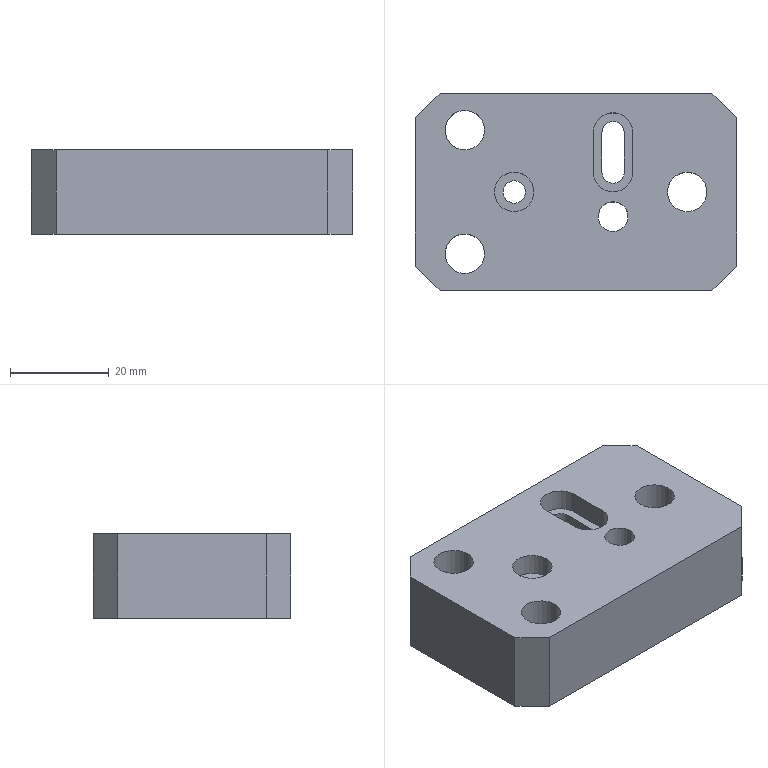Part | SolidWorks | features ICE 4, HoleWzd 3, Chamfer 1, Extrusion 1 | 1 solid | 40 faces | box 65 x 40 x 17 mm | volume 37212 mm3 | cylinder 20 | plane 20 | commonest cylinder face diameters 8 x12 4.5 x4 6 x2 12 x2
STEP:
#1=CARTESIAN_POINT('',(10.5,-5.,8.5));
#2=VERTEX_POINT('',#1);
#3=CARTESIAN_POINT('',(4.5,-5.,8.5));
#4=VERTEX_POINT('',#3);
#5=CARTESIAN_POINT('',(7.5,-5.,8.5));
#6=DIRECTION('',(0.,0.,-1.));
#7=DIRECTION('',(-1.,0.,0.));
#8=AXIS2_PLACEMENT_3D('',#5,#6,#7);
#9=CIRCLE('',#8,3.);
#10=EDGE_CURVE('',#2,#4,#9,.T.);
#11=ORIENTED_EDGE('',*,*,#10,.F.);
#12=CARTESIAN_POINT('',(10.5,-5.,-8.5));
#13=VERTEX_POINT('',#12);
#14=CARTESIAN_POINT('',(10.5,-5.,-8.5));
#15=DIRECTION('',(0.,0.,-1.));
#16=VECTOR('',#15,1000.);
#17=LINE('',#14,#16);
#18=EDGE_CURVE('',#2,#13,#17,.T.);
#19=ORIENTED_EDGE('',*,*,#18,.T.);
#20=CARTESIAN_POINT('',(4.5,-5.,-8.5));
#21=VERTEX_POINT('',#20);
#22=CARTESIAN_POINT('',(7.5,-5.,-8.5));
#23=DIRECTION('',(0.,0.,-1.));
#24=DIRECTION('',(-1.,0.,0.));
#25=AXIS2_PLACEMENT_3D('',#22,#23,#24);
#26=CIRCLE('',#25,3.);
#27=EDGE_CURVE('',#13,#21,#26,.T.);
#28=ORIENTED_EDGE('',*,*,#27,.T.);
#29=CARTESIAN_POINT('',(4.5,-5.,-8.5));
#30=DIRECTION('',(0.,0.,-1.));
#31=VECTOR('',#30,1000.);
#32=LINE('',#29,#31);
#33=EDGE_CURVE('',#4,#21,#32,.T.);
#34=ORIENTED_EDGE('',*,*,#33,.F.);
#35=EDGE_LOOP('',(#11,#19,#28,#34));
#36=FACE_OUTER_BOUND('',#35,.T.);
#37=CARTESIAN_POINT('',(7.5,-5.,-8.5));
#38=DIRECTION('',(0.,0.,-1.));
#39=DIRECTION('',(-1.,0.,0.));
#40=AXIS2_PLACEMENT_3D('',#37,#38,#39);
#41=CYLINDRICAL_SURFACE('',#40,3.);
#42=ADVANCED_FACE('',(#36),#41,.F.);
#43=CARTESIAN_POINT('',(-16.5,0.,4.1));
#44=VERTEX_POINT('',#43);
#45=CARTESIAN_POINT('',(-8.5,0.,4.1));
#46=VERTEX_POINT('',#45);
#47=CARTESIAN_POINT('',(-12.5,0.,4.1));
#48=DIRECTION('',(0.,0.,1.));
#49=DIRECTION('',(1.,0.,0.));
#50=AXIS2_PLACEMENT_3D('',#47,#48,#49);
#51=CIRCLE('',#50,4.);
#52=EDGE_CURVE('',#44,#46,#51,.T.);
#53=ORIENTED_EDGE('',*,*,#52,.F.);
#54=CARTESIAN_POINT('',(-16.5,0.,8.5));
#55=VERTEX_POINT('',#54);
#56=CARTESIAN_POINT('',(-16.5,0.,8.5));
#57=DIRECTION('',(0.,0.,1.));
#58=VECTOR('',#57,1000.);
#59=LINE('',#56,#58);
#60=EDGE_CURVE('',#44,#55,#59,.T.);
#61=ORIENTED_EDGE('',*,*,#60,.T.);
#62=CARTESIAN_POINT('',(-8.5,0.,8.5));
#63=VERTEX_POINT('',#62);
#64=CARTESIAN_POINT('',(-12.5,0.,8.5));
#65=DIRECTION('',(0.,0.,1.));
#66=DIRECTION('',(1.,0.,0.));
#67=AXIS2_PLACEMENT_3D('',#64,#65,#66);
#68=CIRCLE('',#67,4.);
#69=EDGE_CURVE('',#55,#63,#68,.T.);
#70=ORIENTED_EDGE('',*,*,#69,.T.);
#71=CARTESIAN_POINT('',(-8.5,0.,8.5));
#72=DIRECTION('',(0.,0.,1.));
#73=VECTOR('',#72,1000.);
#74=LINE('',#71,#73);
#75=EDGE_CURVE('',#46,#63,#74,.T.);
#76=ORIENTED_EDGE('',*,*,#75,.F.);
#77=EDGE_LOOP('',(#53,#61,#70,#76));
#78=FACE_OUTER_BOUND('',#77,.T.);
#79=CARTESIAN_POINT('',(-12.5,0.,8.5));
#80=DIRECTION('',(0.,0.,1.));
#81=DIRECTION('',(1.,0.,0.));
#82=AXIS2_PLACEMENT_3D('',#79,#80,#81);
#83=CYLINDRICAL_SURFACE('',#82,4.);
#84=ADVANCED_FACE('',(#78),#83,.F.);
#85=CARTESIAN_POINT('',(-10.25,0.,1.));
#86=VERTEX_POINT('',#85);
#87=CARTESIAN_POINT('',(-14.75,0.,1.));
#88=VERTEX_POINT('',#87);
#89=CARTESIAN_POINT('',(-12.5,0.,1.));
#90=DIRECTION('',(0.,0.,-1.));
#91=DIRECTION('',(-1.,0.,0.));
#92=AXIS2_PLACEMENT_3D('',#89,#90,#91);
#93=CIRCLE('',#92,2.25);
#94=EDGE_CURVE('',#86,#88,#93,.T.);
#95=ORIENTED_EDGE('',*,*,#94,.T.);
#96=CARTESIAN_POINT('',(-14.75,0.,4.1));
#97=VERTEX_POINT('',#96);
#98=CARTESIAN_POINT('',(-14.75,0.,8.5));
#99=DIRECTION('',(0.,0.,1.));
#100=VECTOR('',#99,1000.);
#101=LINE('',#98,#100);
#102=EDGE_CURVE('',#88,#97,#101,.T.);
#103=ORIENTED_EDGE('',*,*,#102,.T.);
#104=CARTESIAN_POINT('',(-10.25,0.,4.1));
#105=VERTEX_POINT('',#104);
#106=CARTESIAN_POINT('',(-12.5,0.,4.1));
#107=DIRECTION('',(0.,0.,1.));
#108=DIRECTION('',(1.,0.,0.));
#109=AXIS2_PLACEMENT_3D('',#106,#107,#108);
#110=CIRCLE('',#109,2.25);
#111=EDGE_CURVE('',#97,#105,#110,.T.);
#112=ORIENTED_EDGE('',*,*,#111,.T.);
#113=CARTESIAN_POINT('',(-10.25,0.,8.5));
#114=DIRECTION('',(0.,0.,1.));
#115=VECTOR('',#114,1000.);
#116=LINE('',#113,#115);
#117=EDGE_CURVE('',#86,#105,#116,.T.);
#118=ORIENTED_EDGE('',*,*,#117,.F.);
#119=EDGE_LOOP('',(#95,#103,#112,#118));
#120=FACE_OUTER_BOUND('',#119,.T.);
#121=CARTESIAN_POINT('',(-12.5,0.,8.5));
#122=DIRECTION('',(0.,0.,1.));
#123=DIRECTION('',(1.,0.,0.));
#124=AXIS2_PLACEMENT_3D('',#121,#122,#123);
#125=CYLINDRICAL_SURFACE('',#124,2.25);
#126=ADVANCED_FACE('',(#120),#125,.F.);
#127=CARTESIAN_POINT('',(-6.5,0.,1.));
#128=VERTEX_POINT('',#127);
#129=CARTESIAN_POINT('',(-18.5,0.,1.));
#130=VERTEX_POINT('',#129);
#131=CARTESIAN_POINT('',(-12.5,0.,1.));
#132=DIRECTION('',(0.,0.,-1.));
#133=DIRECTION('',(-1.,0.,0.));
#134=AXIS2_PLACEMENT_3D('',#131,#132,#133);
#135=CIRCLE('',#134,6.);
#136=EDGE_CURVE('',#128,#130,#135,.T.);
#137=ORIENTED_EDGE('',*,*,#136,.F.);
#138=CARTESIAN_POINT('',(-6.5,0.,-8.5));
#139=VERTEX_POINT('',#138);
#140=CARTESIAN_POINT('',(-6.5,0.,1.));
#141=DIRECTION('',(0.,0.,-1.));
#142=VECTOR('',#141,1000.);
#143=LINE('',#140,#142);
#144=EDGE_CURVE('',#128,#139,#143,.T.);
#145=ORIENTED_EDGE('',*,*,#144,.T.);
#146=CARTESIAN_POINT('',(-18.5,0.,-8.5));
#147=VERTEX_POINT('',#146);
#148=CARTESIAN_POINT('',(-12.5,0.,-8.5));
#149=DIRECTION('',(0.,0.,-1.));
#150=DIRECTION('',(-1.,0.,0.));
#151=AXIS2_PLACEMENT_3D('',#148,#149,#150);
#152=CIRCLE('',#151,6.);
#153=EDGE_CURVE('',#139,#147,#152,.T.);
#154=ORIENTED_EDGE('',*,*,#153,.T.);
#155=CARTESIAN_POINT('',(-18.5,0.,1.));
#156=DIRECTION('',(0.,0.,-1.));
#157=VECTOR('',#156,1000.);
#158=LINE('',#155,#157);
#159=EDGE_CURVE('',#130,#147,#158,.T.);
#160=ORIENTED_EDGE('',*,*,#159,.F.);
#161=EDGE_LOOP('',(#137,#145,#154,#160));
#162=FACE_OUTER_BOUND('',#161,.T.);
#163=CARTESIAN_POINT('',(-12.5,0.,1.));
#164=DIRECTION('',(0.,0.,-1.));
#165=DIRECTION('',(-1.,0.,0.));
#166=AXIS2_PLACEMENT_3D('',#163,#164,#165);
#167=CYLINDRICAL_SURFACE('',#166,6.);
#168=ADVANCED_FACE('',(#162),#167,.F.);
#169=CARTESIAN_POINT('',(-26.5,12.5,-8.5));
#170=VERTEX_POINT('',#169);
#171=CARTESIAN_POINT('',(-18.5,12.5,-8.5));
#172=VERTEX_POINT('',#171);
#173=CARTESIAN_POINT('',(-22.5,12.5,-8.5));
#174=DIRECTION('',(0.,0.,1.));
#175=DIRECTION('',(1.,0.,0.));
#176=AXIS2_PLACEMENT_3D('',#173,#174,#175);
#177=CIRCLE('',#176,4.);
#178=EDGE_CURVE('',#170,#172,#177,.T.);
#179=ORIENTED_EDGE('',*,*,#178,.F.);
#180=CARTESIAN_POINT('',(-26.5,12.5,8.5));
#181=VERTEX_POINT('',#180);
#182=CARTESIAN_POINT('',(-26.5,12.5,8.5));
#183=DIRECTION('',(0.,0.,1.));
#184=VECTOR('',#183,1000.);
#185=LINE('',#182,#184);
#186=EDGE_CURVE('',#170,#181,#185,.T.);
#187=ORIENTED_EDGE('',*,*,#186,.T.);
#188=CARTESIAN_POINT('',(-18.5,12.5,8.5));
#189=VERTEX_POINT('',#188);
#190=CARTESIAN_POINT('',(-22.5,12.5,8.5));
#191=DIRECTION('',(0.,0.,1.));
#192=DIRECTION('',(1.,0.,0.));
#193=AXIS2_PLACEMENT_3D('',#190,#191,#192);
#194=CIRCLE('',#193,4.);
#195=EDGE_CURVE('',#181,#189,#194,.T.);
#196=ORIENTED_EDGE('',*,*,#195,.T.);
#197=CARTESIAN_POINT('',(-18.5,12.5,8.5));
#198=DIRECTION('',(0.,0.,1.));
#199=VECTOR('',#198,1000.);
#200=LINE('',#197,#199);
#201=EDGE_CURVE('',#172,#189,#200,.T.);
#202=ORIENTED_EDGE('',*,*,#201,.F.);
#203=EDGE_LOOP('',(#179,#187,#196,#202));
#204=FACE_OUTER_BOUND('',#203,.T.);
#205=CARTESIAN_POINT('',(-22.5,12.5,8.5));
#206=DIRECTION('',(0.,0.,1.));
#207=DIRECTION('',(1.,0.,0.));
#208=AXIS2_PLACEMENT_3D('',#205,#206,#207);
#209=CYLINDRICAL_SURFACE('',#208,4.);
#210=ADVANCED_FACE('',(#204),#209,.F.);
#211=CARTESIAN_POINT('',(-26.5,-12.5,-8.5));
#212=VERTEX_POINT('',#211);
#213=CARTESIAN_POINT('',(-18.5,-12.5,-8.5));
#214=VERTEX_POINT('',#213);
#215=CARTESIAN_POINT('',(-22.5,-12.5,-8.5));
#216=DIRECTION('',(0.,0.,1.));
#217=DIRECTION('',(1.,0.,0.));
#218=AXIS2_PLACEMENT_3D('',#215,#216,#217);
#219=CIRCLE('',#218,4.);
#220=EDGE_CURVE('',#212,#214,#219,.T.);
#221=ORIENTED_EDGE('',*,*,#220,.F.);
#222=CARTESIAN_POINT('',(-26.5,-12.5,8.5));
#223=VERTEX_POINT('',#222);
#224=CARTESIAN_POINT('',(-26.5,-12.5,8.5));
#225=DIRECTION('',(0.,0.,1.));
#226=VECTOR('',#225,1000.);
#227=LINE('',#224,#226);
#228=EDGE_CURVE('',#212,#223,#227,.T.);
#229=ORIENTED_EDGE('',*,*,#228,.T.);
#230=CARTESIAN_POINT('',(-18.5,-12.5,8.5));
#231=VERTEX_POINT('',#230);
#232=CARTESIAN_POINT('',(-22.5,-12.5,8.5));
#233=DIRECTION('',(0.,0.,1.));
#234=DIRECTION('',(1.,0.,0.));
#235=AXIS2_PLACEMENT_3D('',#232,#233,#234);
#236=CIRCLE('',#235,4.);
#237=EDGE_CURVE('',#223,#231,#236,.T.);
#238=ORIENTED_EDGE('',*,*,#237,.T.);
#239=CARTESIAN_POINT('',(-18.5,-12.5,8.5));
#240=DIRECTION('',(0.,0.,1.));
#241=VECTOR('',#240,1000.);
#242=LINE('',#239,#241);
#243=EDGE_CURVE('',#214,#231,#242,.T.);
#244=ORIENTED_EDGE('',*,*,#243,.F.);
#245=EDGE_LOOP('',(#221,#229,#238,#244));
#246=FACE_OUTER_BOUND('',#245,.T.);
#247=CARTESIAN_POINT('',(-22.5,-12.5,8.5));
#248=DIRECTION('',(0.,0.,1.));
#249=DIRECTION('',(1.,0.,0.));
#250=AXIS2_PLACEMENT_3D('',#247,#248,#249);
#251=CYLINDRICAL_SURFACE('',#250,4.);
#252=ADVANCED_FACE('',(#246),#251,.F.);
#253=CARTESIAN_POINT('',(18.5,0.,-8.5));
#254=VERTEX_POINT('',#253);
#255=CARTESIAN_POINT('',(26.5,0.,-8.5));
#256=VERTEX_POINT('',#255);
#257=CARTESIAN_POINT('',(22.5,0.,-8.5));
#258=DIRECTION('',(0.,0.,1.));
#259=DIRECTION('',(1.,0.,0.));
#260=AXIS2_PLACEMENT_3D('',#257,#258,#259);
#261=CIRCLE('',#260,4.);
#262=EDGE_CURVE('',#254,#256,#261,.T.);
#263=ORIENTED_EDGE('',*,*,#262,.F.);
#264=CARTESIAN_POINT('',(18.5,0.,8.5));
#265=VERTEX_POINT('',#264);
#266=CARTESIAN_POINT('',(18.5,0.,8.5));
#267=DIRECTION('',(0.,0.,1.));
#268=VECTOR('',#267,1000.);
#269=LINE('',#266,#268);
#270=EDGE_CURVE('',#254,#265,#269,.T.);
#271=ORIENTED_EDGE('',*,*,#270,.T.);
#272=CARTESIAN_POINT('',(26.5,0.,8.5));
#273=VERTEX_POINT('',#272);
#274=CARTESIAN_POINT('',(22.5,0.,8.5));
#275=DIRECTION('',(0.,0.,1.));
#276=DIRECTION('',(1.,0.,0.));
#277=AXIS2_PLACEMENT_3D('',#274,#275,#276);
#278=CIRCLE('',#277,4.);
#279=EDGE_CURVE('',#265,#273,#278,.T.);
#280=ORIENTED_EDGE('',*,*,#279,.T.);
#281=CARTESIAN_POINT('',(26.5,0.,8.5));
#282=DIRECTION('',(0.,0.,1.));
#283=VECTOR('',#282,1000.);
#284=LINE('',#281,#283);
#285=EDGE_CURVE('',#256,#273,#284,.T.);
#286=ORIENTED_EDGE('',*,*,#285,.F.);
#287=EDGE_LOOP('',(#263,#271,#280,#286));
#288=FACE_OUTER_BOUND('',#287,.T.);
#289=CARTESIAN_POINT('',(22.5,0.,8.5));
#290=DIRECTION('',(0.,0.,1.));
#291=DIRECTION('',(1.,0.,0.));
#292=AXIS2_PLACEMENT_3D('',#289,#290,#291);
#293=CYLINDRICAL_SURFACE('',#292,4.);
#294=ADVANCED_FACE('',(#288),#293,.F.);
#295=CARTESIAN_POINT('',(32.5,-15.,-8.5));
#296=VERTEX_POINT('',#295);
#297=CARTESIAN_POINT('',(32.5,15.,-8.5));
#298=VERTEX_POINT('',#297);
#299=CARTESIAN_POINT('',(32.5,-20.,-8.5));
#300=DIRECTION('',(0.,1.,0.));
#301=VECTOR('',#300,1000.);
#302=LINE('',#299,#301);
#303=EDGE_CURVE('',#296,#298,#302,.T.);
#304=ORIENTED_EDGE('',*,*,#303,.T.);
#305=CARTESIAN_POINT('',(32.5,15.,8.5));
#306=VERTEX_POINT('',#305);
#307=CARTESIAN_POINT('',(32.5,15.,8.5));
#308=DIRECTION('',(0.,0.,1.));
#309=VECTOR('',#308,1000.);
#310=LINE('',#307,#309);
#311=EDGE_CURVE('',#298,#306,#310,.T.);
#312=ORIENTED_EDGE('',*,*,#311,.T.);
#313=CARTESIAN_POINT('',(32.5,-15.,8.5));
#314=VERTEX_POINT('',#313);
#315=CARTESIAN_POINT('',(32.5,-20.,8.5));
#316=DIRECTION('',(0.,1.,0.));
#317=VECTOR('',#316,1000.);
#318=LINE('',#315,#317);
#319=EDGE_CURVE('',#314,#306,#318,.T.);
#320=ORIENTED_EDGE('',*,*,#319,.F.);
#321=CARTESIAN_POINT('',(32.5,-15.,8.5));
#322=DIRECTION('',(0.,0.,-1.));
#323=VECTOR('',#322,1000.);
#324=LINE('',#321,#323);
#325=EDGE_CURVE('',#314,#296,#324,.T.);
#326=ORIENTED_EDGE('',*,*,#325,.T.);
#327=EDGE_LOOP('',(#304,#312,#320,#326));
#328=FACE_OUTER_BOUND('',#327,.T.);
#329=CARTESIAN_POINT('',(32.5,-20.,8.5));
#330=DIRECTION('',(-1.,0.,0.));
#331=DIRECTION('',(0.,0.,1.));
#332=AXIS2_PLACEMENT_3D('',#329,#330,#331);
#333=PLANE('',#332);
#334=ADVANCED_FACE('',(#328),#333,.F.);
#335=CARTESIAN_POINT('',(27.5,20.,-8.5));
#336=VERTEX_POINT('',#335);
#337=CARTESIAN_POINT('',(-27.5,20.,-8.5));
#338=VERTEX_POINT('',#337);
#339=CARTESIAN_POINT('',(-32.5,20.,-8.5));
#340=DIRECTION('',(-1.,0.,0.));
#341=VECTOR('',#340,1000.);
#342=LINE('',#339,#341);
#343=EDGE_CURVE('',#336,#338,#342,.T.);
#344=ORIENTED_EDGE('',*,*,#343,.T.);
#345=CARTESIAN_POINT('',(-27.5,20.,8.5));
#346=VERTEX_POINT('',#345);
#347=CARTESIAN_POINT('',(-27.5,20.,8.5));
#348=DIRECTION('',(0.,0.,1.));
#349=VECTOR('',#348,1000.);
#350=LINE('',#347,#349);
#351=EDGE_CURVE('',#338,#346,#350,.T.);
#352=ORIENTED_EDGE('',*,*,#351,.T.);
#353=CARTESIAN_POINT('',(27.5,20.,8.5));
#354=VERTEX_POINT('',#353);
#355=CARTESIAN_POINT('',(-32.5,20.,8.5));
#356=DIRECTION('',(-1.,0.,0.));
#357=VECTOR('',#356,1000.);
#358=LINE('',#355,#357);
#359=EDGE_CURVE('',#354,#346,#358,.T.);
#360=ORIENTED_EDGE('',*,*,#359,.F.);
#361=CARTESIAN_POINT('',(27.5,20.,8.5));
#362=DIRECTION('',(0.,0.,-1.));
#363=VECTOR('',#362,1000.);
#364=LINE('',#361,#363);
#365=EDGE_CURVE('',#354,#336,#364,.T.);
#366=ORIENTED_EDGE('',*,*,#365,.T.);
#367=EDGE_LOOP('',(#344,#352,#360,#366));
#368=FACE_OUTER_BOUND('',#367,.T.);
#369=CARTESIAN_POINT('',(-32.5,20.,8.5));
#370=DIRECTION('',(0.,-1.,0.));
#371=DIRECTION('',(0.,0.,-1.));
#372=AXIS2_PLACEMENT_3D('',#369,#370,#371);
#373=PLANE('',#372);
#374=ADVANCED_FACE('',(#368),#373,.F.);
#375=CARTESIAN_POINT('',(-32.5,15.,-8.5));
#376=VERTEX_POINT('',#375);
#377=CARTESIAN_POINT('',(-32.5,-15.,-8.5));
#378=VERTEX_POINT('',#377);
#379=CARTESIAN_POINT('',(-32.5,-20.,-8.5));
#380=DIRECTION('',(0.,-1.,0.));
#381=VECTOR('',#380,1000.);
#382=LINE('',#379,#381);
#383=EDGE_CURVE('',#376,#378,#382,.T.);
#384=ORIENTED_EDGE('',*,*,#383,.T.);
#385=CARTESIAN_POINT('',(-32.5,-15.,8.5));
#386=VERTEX_POINT('',#385);
#387=CARTESIAN_POINT('',(-32.5,-15.,8.5));
#388=DIRECTION('',(0.,0.,1.));
#389=VECTOR('',#388,1000.);
#390=LINE('',#387,#389);
#391=EDGE_CURVE('',#378,#386,#390,.T.);
#392=ORIENTED_EDGE('',*,*,#391,.T.);
#393=CARTESIAN_POINT('',(-32.5,15.,8.5));
#394=VERTEX_POINT('',#393);
#395=CARTESIAN_POINT('',(-32.5,-20.,8.5));
#396=DIRECTION('',(0.,-1.,0.));
#397=VECTOR('',#396,1000.);
#398=LINE('',#395,#397);
#399=EDGE_CURVE('',#394,#386,#398,.T.);
#400=ORIENTED_EDGE('',*,*,#399,.F.);
#401=CARTESIAN_POINT('',(-32.5,15.,8.5));
#402=DIRECTION('',(0.,0.,-1.));
#403=VECTOR('',#402,1000.);
#404=LINE('',#401,#403);
#405=EDGE_CURVE('',#394,#376,#404,.T.);
#406=ORIENTED_EDGE('',*,*,#405,.T.);
#407=EDGE_LOOP('',(#384,#392,#400,#406));
#408=FACE_OUTER_BOUND('',#407,.T.);
#409=CARTESIAN_POINT('',(-32.5,-20.,8.5));
#410=DIRECTION('',(1.,0.,0.));
#411=DIRECTION('',(0.,0.,-1.));
#412=AXIS2_PLACEMENT_3D('',#409,#410,#411);
#413=PLANE('',#412);
#414=ADVANCED_FACE('',(#408),#413,.F.);
#415=CARTESIAN_POINT('',(-27.5,-20.,8.5));
#416=VERTEX_POINT('',#415);
#417=CARTESIAN_POINT('',(27.5,-20.,8.5));
#418=VERTEX_POINT('',#417);
#419=CARTESIAN_POINT('',(-32.5,-20.,8.5));
#420=DIRECTION('',(1.,0.,0.));
#421=VECTOR('',#420,1000.);
#422=LINE('',#419,#421);
#423=EDGE_CURVE('',#416,#418,#422,.T.);
#424=ORIENTED_EDGE('',*,*,#423,.F.);
#425=CARTESIAN_POINT('',(-27.5,-20.,-8.5));
#426=VERTEX_POINT('',#425);
#427=CARTESIAN_POINT('',(-27.5,-20.,8.5));
#428=DIRECTION('',(0.,0.,-1.));
#429=VECTOR('',#428,1000.);
#430=LINE('',#427,#429);
#431=EDGE_CURVE('',#416,#426,#430,.T.);
#432=ORIENTED_EDGE('',*,*,#431,.T.);
#433=CARTESIAN_POINT('',(27.5,-20.,-8.5));
#434=VERTEX_POINT('',#433);
#435=CARTESIAN_POINT('',(-32.5,-20.,-8.5));
#436=DIRECTION('',(1.,0.,0.));
#437=VECTOR('',#436,1000.);
#438=LINE('',#435,#437);
#439=EDGE_CURVE('',#426,#434,#438,.T.);
#440=ORIENTED_EDGE('',*,*,#439,.T.);
#441=CARTESIAN_POINT('',(27.5,-20.,8.5));
#442=DIRECTION('',(0.,0.,1.));
#443=VECTOR('',#442,1000.);
#444=LINE('',#441,#443);
#445=EDGE_CURVE('',#434,#418,#444,.T.);
#446=ORIENTED_EDGE('',*,*,#445,.T.);
#447=EDGE_LOOP('',(#424,#432,#440,#446));
#448=FACE_OUTER_BOUND('',#447,.T.);
#449=CARTESIAN_POINT('',(-32.5,-20.,8.5));
#450=DIRECTION('',(0.,1.,0.));
#451=DIRECTION('',(0.,0.,1.));
#452=AXIS2_PLACEMENT_3D('',#449,#450,#451);
#453=PLANE('',#452);
#454=ADVANCED_FACE('',(#448),#453,.F.);
#455=CARTESIAN_POINT('',(11.5,12.,8.5));
#456=VERTEX_POINT('',#455);
#457=CARTESIAN_POINT('',(3.5,12.,8.5));
#458=VERTEX_POINT('',#457);
#459=CARTESIAN_POINT('',(7.5,12.,8.5));
#460=DIRECTION('',(0.,0.,1.));
#461=DIRECTION('',(1.,0.,0.));
#462=AXIS2_PLACEMENT_3D('',#459,#460,#461);
#463=CIRCLE('',#462,4.);
#464=EDGE_CURVE('',#456,#458,#463,.T.);
#465=ORIENTED_EDGE('',*,*,#464,.F.);
#466=CARTESIAN_POINT('',(11.5,4.,8.5));
#467=VERTEX_POINT('',#466);
#468=CARTESIAN_POINT('',(11.5,4.,8.5));
#469=DIRECTION('',(0.,1.,0.));
#470=VECTOR('',#469,1000.);
#471=LINE('',#468,#470);
#472=EDGE_CURVE('',#467,#456,#471,.T.);
#473=ORIENTED_EDGE('',*,*,#472,.F.);
#474=CARTESIAN_POINT('',(3.5,4.,8.5));
#475=VERTEX_POINT('',#474);
#476=CARTESIAN_POINT('',(7.5,4.,8.5));
#477=DIRECTION('',(0.,0.,1.));
#478=DIRECTION('',(1.,0.,0.));
#479=AXIS2_PLACEMENT_3D('',#476,#477,#478);
#480=CIRCLE('',#479,4.);
#481=EDGE_CURVE('',#475,#467,#480,.T.);
#482=ORIENTED_EDGE('',*,*,#481,.F.);
#483=CARTESIAN_POINT('',(3.5,4.,8.5));
#484=DIRECTION('',(0.,-1.,0.));
#485=VECTOR('',#484,1000.);
#486=LINE('',#483,#485);
#487=EDGE_CURVE('',#458,#475,#486,.T.);
#488=ORIENTED_EDGE('',*,*,#487,.F.);
#489=EDGE_LOOP('',(#465,#473,#482,#488));
#490=FACE_BOUND('',#489,.T.);
#491=CARTESIAN_POINT('',(7.5,-5.,8.5));
#492=DIRECTION('',(0.,0.,-1.));
#493=DIRECTION('',(-1.,0.,0.));
#494=AXIS2_PLACEMENT_3D('',#491,#492,#493);
#495=CIRCLE('',#494,3.);
#496=EDGE_CURVE('',#4,#2,#495,.T.);
#497=ORIENTED_EDGE('',*,*,#496,.T.);
#498=ORIENTED_EDGE('',*,*,#10,.T.);
#499=EDGE_LOOP('',(#497,#498));
#500=FACE_BOUND('',#499,.T.);
#501=CARTESIAN_POINT('',(-12.5,0.,8.5));
#502=DIRECTION('',(0.,0.,1.));
#503=DIRECTION('',(1.,0.,0.));
#504=AXIS2_PLACEMENT_3D('',#501,#502,#503);
#505=CIRCLE('',#504,4.);
#506=EDGE_CURVE('',#63,#55,#505,.T.);
#507=ORIENTED_EDGE('',*,*,#506,.F.);
#508=ORIENTED_EDGE('',*,*,#69,.F.);
#509=EDGE_LOOP('',(#507,#508));
#510=FACE_BOUND('',#509,.T.);
#511=CARTESIAN_POINT('',(-22.5,12.5,8.5));
#512=DIRECTION('',(0.,0.,1.));
#513=DIRECTION('',(1.,0.,0.));
#514=AXIS2_PLACEMENT_3D('',#511,#512,#513);
#515=CIRCLE('',#514,4.);
#516=EDGE_CURVE('',#189,#181,#515,.T.);
#517=ORIENTED_EDGE('',*,*,#516,.F.);
#518=ORIENTED_EDGE('',*,*,#195,.F.);
#519=EDGE_LOOP('',(#517,#518));
#520=FACE_BOUND('',#519,.T.);
#521=CARTESIAN_POINT('',(-22.5,-12.5,8.5));
#522=DIRECTION('',(0.,0.,1.));
#523=DIRECTION('',(1.,0.,0.));
#524=AXIS2_PLACEMENT_3D('',#521,#522,#523);
#525=CIRCLE('',#524,4.);
#526=EDGE_CURVE('',#231,#223,#525,.T.);
#527=ORIENTED_EDGE('',*,*,#526,.F.);
#528=ORIENTED_EDGE('',*,*,#237,.F.);
#529=EDGE_LOOP('',(#527,#528));
#530=FACE_BOUND('',#529,.T.);
#531=CARTESIAN_POINT('',(22.5,0.,8.5));
#532=DIRECTION('',(0.,0.,1.));
#533=DIRECTION('',(1.,0.,0.));
#534=AXIS2_PLACEMENT_3D('',#531,#532,#533);
#535=CIRCLE('',#534,4.);
#536=EDGE_CURVE('',#273,#265,#535,.T.);
#537=ORIENTED_EDGE('',*,*,#536,.F.);
#538=ORIENTED_EDGE('',*,*,#279,.F.);
#539=EDGE_LOOP('',(#537,#538));
#540=FACE_BOUND('',#539,.T.);
#541=ORIENTED_EDGE('',*,*,#399,.T.);
#542=CARTESIAN_POINT('',(-27.5,-20.,8.5));
#543=DIRECTION('',(0.7071,-0.7071,0.));
#544=VECTOR('',#543,1000.);
#545=LINE('',#542,#544);
#546=EDGE_CURVE('',#386,#416,#545,.T.);
#547=ORIENTED_EDGE('',*,*,#546,.T.);
#548=ORIENTED_EDGE('',*,*,#423,.T.);
#549=CARTESIAN_POINT('',(32.5,-15.,8.5));
#550=DIRECTION('',(0.7071,0.7071,0.));
#551=VECTOR('',#550,1000.);
#552=LINE('',#549,#551);
#553=EDGE_CURVE('',#418,#314,#552,.T.);
#554=ORIENTED_EDGE('',*,*,#553,.T.);
#555=ORIENTED_EDGE('',*,*,#319,.T.);
#556=CARTESIAN_POINT('',(27.5,20.,8.5));
#557=DIRECTION('',(-0.7071,0.7071,0.));
#558=VECTOR('',#557,1000.);
#559=LINE('',#556,#558);
#560=EDGE_CURVE('',#306,#354,#559,.T.);
#561=ORIENTED_EDGE('',*,*,#560,.T.);
#562=ORIENTED_EDGE('',*,*,#359,.T.);
#563=CARTESIAN_POINT('',(-32.5,15.,8.5));
#564=DIRECTION('',(-0.7071,-0.7071,0.));
#565=VECTOR('',#564,1000.);
#566=LINE('',#563,#565);
#567=EDGE_CURVE('',#346,#394,#566,.T.);
#568=ORIENTED_EDGE('',*,*,#567,.T.);
#569=EDGE_LOOP('',(#541,#547,#548,#554,#555,#561,#562,#568));
#570=FACE_OUTER_BOUND('',#569,.T.);
#571=CARTESIAN_POINT('',(0.,0.,8.5));
#572=DIRECTION('',(0.,0.,-1.));
#573=DIRECTION('',(-1.,0.,0.));
#574=AXIS2_PLACEMENT_3D('',#571,#572,#573);
#575=PLANE('',#574);
#576=ADVANCED_FACE('',(#490,#500,#510,#520,#530,#540,#570),#575,.F.);
#577=CARTESIAN_POINT('',(11.5,4.,-8.5));
#578=VERTEX_POINT('',#577);
#579=CARTESIAN_POINT('',(3.5,4.,-8.5));
#580=VERTEX_POINT('',#579);
#581=CARTESIAN_POINT('',(7.5,4.,-8.5));
#582=DIRECTION('',(0.,0.,-1.));
#583=DIRECTION('',(-1.,0.,0.));
#584=AXIS2_PLACEMENT_3D('',#581,#582,#583);
#585=CIRCLE('',#584,4.);
#586=EDGE_CURVE('',#578,#580,#585,.T.);
#587=ORIENTED_EDGE('',*,*,#586,.F.);
#588=CARTESIAN_POINT('',(11.5,12.,-8.5));
#589=VERTEX_POINT('',#588);
#590=CARTESIAN_POINT('',(11.5,4.,-8.5));
#591=DIRECTION('',(0.,-1.,0.));
#592=VECTOR('',#591,1000.);
#593=LINE('',#590,#592);
#594=EDGE_CURVE('',#589,#578,#593,.T.);
#595=ORIENTED_EDGE('',*,*,#594,.F.);
#596=CARTESIAN_POINT('',(3.5,12.,-8.5));
#597=VERTEX_POINT('',#596);
#598=CARTESIAN_POINT('',(7.5,12.,-8.5));
#599=DIRECTION('',(0.,0.,-1.));
#600=DIRECTION('',(-1.,0.,0.));
#601=AXIS2_PLACEMENT_3D('',#598,#599,#600);
#602=CIRCLE('',#601,4.);
#603=EDGE_CURVE('',#597,#589,#602,.T.);
#604=ORIENTED_EDGE('',*,*,#603,.F.);
#605=CARTESIAN_POINT('',(3.5,4.,-8.5));
#606=DIRECTION('',(0.,1.,0.));
#607=VECTOR('',#606,1000.);
#608=LINE('',#605,#607);
#609=EDGE_CURVE('',#580,#597,#608,.T.);
#610=ORIENTED_EDGE('',*,*,#609,.F.);
#611=EDGE_LOOP('',(#587,#595,#604,#610));
#612=FACE_BOUND('',#611,.T.);
#613=CARTESIAN_POINT('',(7.5,-5.,-8.5));
#614=DIRECTION('',(0.,0.,-1.));
#615=DIRECTION('',(-1.,0.,0.));
#616=AXIS2_PLACEMENT_3D('',#613,#614,#615);
#617=CIRCLE('',#616,3.);
#618=EDGE_CURVE('',#21,#13,#617,.T.);
#619=ORIENTED_EDGE('',*,*,#618,.F.);
#620=ORIENTED_EDGE('',*,*,#27,.F.);
#621=EDGE_LOOP('',(#619,#620));
#622=FACE_BOUND('',#621,.T.);
#623=CARTESIAN_POINT('',(-12.5,0.,-8.5));
#624=DIRECTION('',(0.,0.,-1.));
#625=DIRECTION('',(-1.,0.,0.));
#626=AXIS2_PLACEMENT_3D('',#623,#624,#625);
#627=CIRCLE('',#626,6.);
#628=EDGE_CURVE('',#147,#139,#627,.T.);
#629=ORIENTED_EDGE('',*,*,#628,.F.);
#630=ORIENTED_EDGE('',*,*,#153,.F.);
#631=EDGE_LOOP('',(#629,#630));
#632=FACE_BOUND('',#631,.T.);
#633=CARTESIAN_POINT('',(-22.5,12.5,-8.5));
#634=DIRECTION('',(0.,0.,1.));
#635=DIRECTION('',(1.,0.,0.));
#636=AXIS2_PLACEMENT_3D('',#633,#634,#635);
#637=CIRCLE('',#636,4.);
#638=EDGE_CURVE('',#172,#170,#637,.T.);
#639=ORIENTED_EDGE('',*,*,#638,.T.);
#640=ORIENTED_EDGE('',*,*,#178,.T.);
#641=EDGE_LOOP('',(#639,#640));
#642=FACE_BOUND('',#641,.T.);
#643=CARTESIAN_POINT('',(-22.5,-12.5,-8.5));
#644=DIRECTION('',(0.,0.,1.));
#645=DIRECTION('',(1.,0.,0.));
#646=AXIS2_PLACEMENT_3D('',#643,#644,#645);
#647=CIRCLE('',#646,4.);
#648=EDGE_CURVE('',#214,#212,#647,.T.);
#649=ORIENTED_EDGE('',*,*,#648,.T.);
#650=ORIENTED_EDGE('',*,*,#220,.T.);
#651=EDGE_LOOP('',(#649,#650));
#652=FACE_BOUND('',#651,.T.);
#653=CARTESIAN_POINT('',(22.5,0.,-8.5));
#654=DIRECTION('',(0.,0.,1.));
#655=DIRECTION('',(1.,0.,0.));
#656=AXIS2_PLACEMENT_3D('',#653,#654,#655);
#657=CIRCLE('',#656,4.);
#658=EDGE_CURVE('',#256,#254,#657,.T.);
#659=ORIENTED_EDGE('',*,*,#658,.T.);
#660=ORIENTED_EDGE('',*,*,#262,.T.);
#661=EDGE_LOOP('',(#659,#660));
#662=FACE_BOUND('',#661,.T.);
#663=ORIENTED_EDGE('',*,*,#439,.F.);
#664=CARTESIAN_POINT('',(-23.75,-23.75,-8.5));
#665=DIRECTION('',(-0.7071,0.7071,0.));
#666=VECTOR('',#665,1000.);
#667=LINE('',#664,#666);
#668=EDGE_CURVE('',#426,#378,#667,.T.);
#669=ORIENTED_EDGE('',*,*,#668,.T.);
#670=ORIENTED_EDGE('',*,*,#383,.F.);
#671=CARTESIAN_POINT('',(-23.75,23.75,-8.5));
#672=DIRECTION('',(0.7071,0.7071,0.));
#673=VECTOR('',#672,1000.);
#674=LINE('',#671,#673);
#675=EDGE_CURVE('',#376,#338,#674,.T.);
#676=ORIENTED_EDGE('',*,*,#675,.T.);
#677=ORIENTED_EDGE('',*,*,#343,.F.);
#678=CARTESIAN_POINT('',(23.75,23.75,-8.5));
#679=DIRECTION('',(0.7071,-0.7071,0.));
#680=VECTOR('',#679,1000.);
#681=LINE('',#678,#680);
#682=EDGE_CURVE('',#336,#298,#681,.T.);
#683=ORIENTED_EDGE('',*,*,#682,.T.);
#684=ORIENTED_EDGE('',*,*,#303,.F.);
#685=CARTESIAN_POINT('',(23.75,-23.75,-8.5));
#686=DIRECTION('',(-0.7071,-0.7071,0.));
#687=VECTOR('',#686,1000.);
#688=LINE('',#685,#687);
#689=EDGE_CURVE('',#296,#434,#688,.T.);
#690=ORIENTED_EDGE('',*,*,#689,.T.);
#691=EDGE_LOOP('',(#663,#669,#670,#676,#677,#683,#684,#690));
#692=FACE_OUTER_BOUND('',#691,.T.);
#693=CARTESIAN_POINT('',(0.,0.,-8.5));
#694=DIRECTION('',(0.,0.,-1.));
#695=DIRECTION('',(-1.,0.,0.));
#696=AXIS2_PLACEMENT_3D('',#693,#694,#695);
#697=PLANE('',#696);
#698=ADVANCED_FACE('',(#612,#622,#632,#642,#652,#662,#692),#697,.T.);
#699=ORIENTED_EDGE('',*,*,#270,.F.);
#700=ORIENTED_EDGE('',*,*,#658,.F.);
#701=ORIENTED_EDGE('',*,*,#285,.T.);
#702=ORIENTED_EDGE('',*,*,#536,.T.);
#703=EDGE_LOOP('',(#699,#700,#701,#702));
#704=FACE_OUTER_BOUND('',#703,.T.);
#705=CARTESIAN_POINT('',(22.5,0.,8.5));
#706=DIRECTION('',(0.,0.,1.));
#707=DIRECTION('',(1.,0.,0.));
#708=AXIS2_PLACEMENT_3D('',#705,#706,#707);
#709=CYLINDRICAL_SURFACE('',#708,4.);
#710=ADVANCED_FACE('',(#704),#709,.F.);
#711=ORIENTED_EDGE('',*,*,#228,.F.);
#712=ORIENTED_EDGE('',*,*,#648,.F.);
#713=ORIENTED_EDGE('',*,*,#243,.T.);
#714=ORIENTED_EDGE('',*,*,#526,.T.);
#715=EDGE_LOOP('',(#711,#712,#713,#714));
#716=FACE_OUTER_BOUND('',#715,.T.);
#717=CARTESIAN_POINT('',(-22.5,-12.5,8.5));
#718=DIRECTION('',(0.,0.,1.));
#719=DIRECTION('',(1.,0.,0.));
#720=AXIS2_PLACEMENT_3D('',#717,#718,#719);
#721=CYLINDRICAL_SURFACE('',#720,4.);
#722=ADVANCED_FACE('',(#716),#721,.F.);
#723=ORIENTED_EDGE('',*,*,#186,.F.);
#724=ORIENTED_EDGE('',*,*,#638,.F.);
#725=ORIENTED_EDGE('',*,*,#201,.T.);
#726=ORIENTED_EDGE('',*,*,#516,.T.);
#727=EDGE_LOOP('',(#723,#724,#725,#726));
#728=FACE_OUTER_BOUND('',#727,.T.);
#729=CARTESIAN_POINT('',(-22.5,12.5,8.5));
#730=DIRECTION('',(0.,0.,1.));
#731=DIRECTION('',(1.,0.,0.));
#732=AXIS2_PLACEMENT_3D('',#729,#730,#731);
#733=CYLINDRICAL_SURFACE('',#732,4.);
#734=ADVANCED_FACE('',(#728),#733,.F.);
#735=ORIENTED_EDGE('',*,*,#144,.F.);
#736=CARTESIAN_POINT('',(-12.5,0.,1.));
#737=DIRECTION('',(0.,0.,-1.));
#738=DIRECTION('',(-1.,0.,0.));
#739=AXIS2_PLACEMENT_3D('',#736,#737,#738);
#740=CIRCLE('',#739,6.);
#741=EDGE_CURVE('',#130,#128,#740,.T.);
#742=ORIENTED_EDGE('',*,*,#741,.F.);
#743=ORIENTED_EDGE('',*,*,#159,.T.);
#744=ORIENTED_EDGE('',*,*,#628,.T.);
#745=EDGE_LOOP('',(#735,#742,#743,#744));
#746=FACE_OUTER_BOUND('',#745,.T.);
#747=CARTESIAN_POINT('',(-12.5,0.,1.));
#748=DIRECTION('',(0.,0.,-1.));
#749=DIRECTION('',(-1.,0.,0.));
#750=AXIS2_PLACEMENT_3D('',#747,#748,#749);
#751=CYLINDRICAL_SURFACE('',#750,6.);
#752=ADVANCED_FACE('',(#746),#751,.F.);
#753=ORIENTED_EDGE('',*,*,#94,.F.);
#754=CARTESIAN_POINT('',(-12.5,0.,1.));
#755=DIRECTION('',(0.,0.,-1.));
#756=DIRECTION('',(-1.,0.,0.));
#757=AXIS2_PLACEMENT_3D('',#754,#755,#756);
#758=CIRCLE('',#757,2.25);
#759=EDGE_CURVE('',#88,#86,#758,.T.);
#760=ORIENTED_EDGE('',*,*,#759,.F.);
#761=EDGE_LOOP('',(#753,#760));
#762=FACE_BOUND('',#761,.T.);
#763=ORIENTED_EDGE('',*,*,#741,.T.);
#764=ORIENTED_EDGE('',*,*,#136,.T.);
#765=EDGE_LOOP('',(#763,#764));
#766=FACE_OUTER_BOUND('',#765,.T.);
#767=CARTESIAN_POINT('',(-12.5,0.,1.));
#768=DIRECTION('',(0.,0.,-1.));
#769=DIRECTION('',(-1.,0.,0.));
#770=AXIS2_PLACEMENT_3D('',#767,#768,#769);
#771=PLANE('',#770);
#772=ADVANCED_FACE('',(#762,#766),#771,.T.);
#773=ORIENTED_EDGE('',*,*,#102,.F.);
#774=ORIENTED_EDGE('',*,*,#759,.T.);
#775=ORIENTED_EDGE('',*,*,#117,.T.);
#776=CARTESIAN_POINT('',(-12.5,0.,4.1));
#777=DIRECTION('',(0.,0.,1.));
#778=DIRECTION('',(1.,0.,0.));
#779=AXIS2_PLACEMENT_3D('',#776,#777,#778);
#780=CIRCLE('',#779,2.25);
#781=EDGE_CURVE('',#105,#97,#780,.T.);
#782=ORIENTED_EDGE('',*,*,#781,.T.);
#783=EDGE_LOOP('',(#773,#774,#775,#782));
#784=FACE_OUTER_BOUND('',#783,.T.);
#785=CARTESIAN_POINT('',(-12.5,0.,8.5));
#786=DIRECTION('',(0.,0.,1.));
#787=DIRECTION('',(1.,0.,0.));
#788=AXIS2_PLACEMENT_3D('',#785,#786,#787);
#789=CYLINDRICAL_SURFACE('',#788,2.25);
#790=ADVANCED_FACE('',(#784),#789,.F.);
#791=ORIENTED_EDGE('',*,*,#781,.F.);
#792=ORIENTED_EDGE('',*,*,#111,.F.);
#793=EDGE_LOOP('',(#791,#792));
#794=FACE_BOUND('',#793,.T.);
#795=CARTESIAN_POINT('',(-12.5,0.,4.1));
#796=DIRECTION('',(0.,0.,1.));
#797=DIRECTION('',(1.,0.,0.));
#798=AXIS2_PLACEMENT_3D('',#795,#796,#797);
#799=CIRCLE('',#798,4.);
#800=EDGE_CURVE('',#46,#44,#799,.T.);
#801=ORIENTED_EDGE('',*,*,#800,.T.);
#802=ORIENTED_EDGE('',*,*,#52,.T.);
#803=EDGE_LOOP('',(#801,#802));
#804=FACE_OUTER_BOUND('',#803,.T.);
#805=CARTESIAN_POINT('',(-10.25,0.,4.1));
#806=DIRECTION('',(0.,0.,-1.));
#807=DIRECTION('',(-1.,0.,0.));
#808=AXIS2_PLACEMENT_3D('',#805,#806,#807);
#809=PLANE('',#808);
#810=ADVANCED_FACE('',(#794,#804),#809,.F.);
#811=ORIENTED_EDGE('',*,*,#60,.F.);
#812=ORIENTED_EDGE('',*,*,#800,.F.);
#813=ORIENTED_EDGE('',*,*,#75,.T.);
#814=ORIENTED_EDGE('',*,*,#506,.T.);
#815=EDGE_LOOP('',(#811,#812,#813,#814));
#816=FACE_OUTER_BOUND('',#815,.T.);
#817=CARTESIAN_POINT('',(-12.5,0.,8.5));
#818=DIRECTION('',(0.,0.,1.));
#819=DIRECTION('',(1.,0.,0.));
#820=AXIS2_PLACEMENT_3D('',#817,#818,#819);
#821=CYLINDRICAL_SURFACE('',#820,4.);
#822=ADVANCED_FACE('',(#816),#821,.F.);
#823=ORIENTED_EDGE('',*,*,#18,.F.);
#824=ORIENTED_EDGE('',*,*,#496,.F.);
#825=ORIENTED_EDGE('',*,*,#33,.T.);
#826=ORIENTED_EDGE('',*,*,#618,.T.);
#827=EDGE_LOOP('',(#823,#824,#825,#826));
#828=FACE_OUTER_BOUND('',#827,.T.);
#829=CARTESIAN_POINT('',(7.5,-5.,-8.5));
#830=DIRECTION('',(0.,0.,-1.));
#831=DIRECTION('',(-1.,0.,0.));
#832=AXIS2_PLACEMENT_3D('',#829,#830,#831);
#833=CYLINDRICAL_SURFACE('',#832,3.);
#834=ADVANCED_FACE('',(#828),#833,.F.);
#835=CARTESIAN_POINT('',(3.5,4.,1.));
#836=VERTEX_POINT('',#835);
#837=CARTESIAN_POINT('',(11.5,4.,1.));
#838=VERTEX_POINT('',#837);
#839=CARTESIAN_POINT('',(7.5,4.,1.));
#840=DIRECTION('',(0.,0.,1.));
#841=DIRECTION('',(-1.,0.,0.));
#842=AXIS2_PLACEMENT_3D('',#839,#840,#841);
#843=CIRCLE('',#842,4.);
#844=EDGE_CURVE('',#836,#838,#843,.T.);
#845=ORIENTED_EDGE('',*,*,#844,.T.);
#846=CARTESIAN_POINT('',(11.5,4.,18.889));
#847=DIRECTION('',(0.,0.,-1.));
#848=VECTOR('',#847,1000.);
#849=LINE('',#846,#848);
#850=EDGE_CURVE('',#838,#578,#849,.T.);
#851=ORIENTED_EDGE('',*,*,#850,.T.);
#852=ORIENTED_EDGE('',*,*,#586,.T.);
#853=CARTESIAN_POINT('',(3.5,4.,18.889));
#854=DIRECTION('',(0.,0.,-1.));
#855=VECTOR('',#854,1000.);
#856=LINE('',#853,#855);
#857=EDGE_CURVE('',#836,#580,#856,.T.);
#858=ORIENTED_EDGE('',*,*,#857,.F.);
#859=EDGE_LOOP('',(#845,#851,#852,#858));
#860=FACE_OUTER_BOUND('',#859,.T.);
#861=CARTESIAN_POINT('',(7.5,4.,18.889));
#862=DIRECTION('',(0.,0.,-1.));
#863=DIRECTION('',(-1.,0.,0.));
#864=AXIS2_PLACEMENT_3D('',#861,#862,#863);
#865=CYLINDRICAL_SURFACE('',#864,4.);
#866=ADVANCED_FACE('',(#860),#865,.F.);
#867=CARTESIAN_POINT('',(11.5,12.,1.));
#868=VERTEX_POINT('',#867);
#869=CARTESIAN_POINT('',(11.5,4.,1.));
#870=DIRECTION('',(0.,1.,0.));
#871=VECTOR('',#870,1000.);
#872=LINE('',#869,#871);
#873=EDGE_CURVE('',#838,#868,#872,.T.);
#874=ORIENTED_EDGE('',*,*,#873,.T.);
#875=CARTESIAN_POINT('',(11.5,12.,18.889));
#876=DIRECTION('',(0.,0.,-1.));
#877=VECTOR('',#876,1000.);
#878=LINE('',#875,#877);
#879=EDGE_CURVE('',#868,#589,#878,.T.);
#880=ORIENTED_EDGE('',*,*,#879,.T.);
#881=ORIENTED_EDGE('',*,*,#594,.T.);
#882=ORIENTED_EDGE('',*,*,#850,.F.);
#883=EDGE_LOOP('',(#874,#880,#881,#882));
#884=FACE_OUTER_BOUND('',#883,.T.);
#885=CARTESIAN_POINT('',(11.5,4.,18.889));
#886=DIRECTION('',(1.,0.,0.));
#887=DIRECTION('',(0.,1.,0.));
#888=AXIS2_PLACEMENT_3D('',#885,#886,#887);
#889=PLANE('',#888);
#890=ADVANCED_FACE('',(#884),#889,.F.);
#891=CARTESIAN_POINT('',(3.5,12.,1.));
#892=VERTEX_POINT('',#891);
#893=CARTESIAN_POINT('',(7.5,12.,1.));
#894=DIRECTION('',(0.,0.,1.));
#895=DIRECTION('',(-1.,0.,0.));
#896=AXIS2_PLACEMENT_3D('',#893,#894,#895);
#897=CIRCLE('',#896,4.);
#898=EDGE_CURVE('',#868,#892,#897,.T.);
#899=ORIENTED_EDGE('',*,*,#898,.T.);
#900=CARTESIAN_POINT('',(3.5,12.,18.889));
#901=DIRECTION('',(0.,0.,-1.));
#902=VECTOR('',#901,1000.);
#903=LINE('',#900,#902);
#904=EDGE_CURVE('',#892,#597,#903,.T.);
#905=ORIENTED_EDGE('',*,*,#904,.T.);
#906=ORIENTED_EDGE('',*,*,#603,.T.);
#907=ORIENTED_EDGE('',*,*,#879,.F.);
#908=EDGE_LOOP('',(#899,#905,#906,#907));
#909=FACE_OUTER_BOUND('',#908,.T.);
#910=CARTESIAN_POINT('',(7.5,12.,18.889));
#911=DIRECTION('',(0.,0.,-1.));
#912=DIRECTION('',(-1.,0.,0.));
#913=AXIS2_PLACEMENT_3D('',#910,#911,#912);
#914=CYLINDRICAL_SURFACE('',#913,4.);
#915=ADVANCED_FACE('',(#909),#914,.F.);
#916=CARTESIAN_POINT('',(3.5,4.,1.));
#917=DIRECTION('',(0.,-1.,0.));
#918=VECTOR('',#917,1000.);
#919=LINE('',#916,#918);
#920=EDGE_CURVE('',#892,#836,#919,.T.);
#921=ORIENTED_EDGE('',*,*,#920,.T.);
#922=ORIENTED_EDGE('',*,*,#857,.T.);
#923=ORIENTED_EDGE('',*,*,#609,.T.);
#924=ORIENTED_EDGE('',*,*,#904,.F.);
#925=EDGE_LOOP('',(#921,#922,#923,#924));
#926=FACE_OUTER_BOUND('',#925,.T.);
#927=CARTESIAN_POINT('',(3.5,4.,18.889));
#928=DIRECTION('',(-1.,0.,0.));
#929=DIRECTION('',(0.,0.,1.));
#930=AXIS2_PLACEMENT_3D('',#927,#928,#929);
#931=PLANE('',#930);
#932=ADVANCED_FACE('',(#926),#931,.F.);
#933=CARTESIAN_POINT('',(9.75,4.,1.));
#934=VERTEX_POINT('',#933);
#935=CARTESIAN_POINT('',(5.25,4.,1.));
#936=VERTEX_POINT('',#935);
#937=CARTESIAN_POINT('',(7.5,4.,1.));
#938=DIRECTION('',(0.,0.,-1.));
#939=DIRECTION('',(-1.,0.,0.));
#940=AXIS2_PLACEMENT_3D('',#937,#938,#939);
#941=CIRCLE('',#940,2.25);
#942=EDGE_CURVE('',#934,#936,#941,.T.);
#943=ORIENTED_EDGE('',*,*,#942,.F.);
#944=CARTESIAN_POINT('',(9.75,12.,1.));
#945=VERTEX_POINT('',#944);
#946=CARTESIAN_POINT('',(9.75,0.,1.));
#947=DIRECTION('',(0.,-1.,0.));
#948=VECTOR('',#947,1000.);
#949=LINE('',#946,#948);
#950=EDGE_CURVE('',#945,#934,#949,.T.);
#951=ORIENTED_EDGE('',*,*,#950,.F.);
#952=CARTESIAN_POINT('',(5.25,12.,1.));
#953=VERTEX_POINT('',#952);
#954=CARTESIAN_POINT('',(7.5,12.,1.));
#955=DIRECTION('',(0.,0.,-1.));
#956=DIRECTION('',(-1.,0.,0.));
#957=AXIS2_PLACEMENT_3D('',#954,#955,#956);
#958=CIRCLE('',#957,2.25);
#959=EDGE_CURVE('',#953,#945,#958,.T.);
#960=ORIENTED_EDGE('',*,*,#959,.F.);
#961=CARTESIAN_POINT('',(5.25,0.,1.));
#962=DIRECTION('',(0.,1.,0.));
#963=VECTOR('',#962,1000.);
#964=LINE('',#961,#963);
#965=EDGE_CURVE('',#936,#953,#964,.T.);
#966=ORIENTED_EDGE('',*,*,#965,.F.);
#967=EDGE_LOOP('',(#943,#951,#960,#966));
#968=FACE_BOUND('',#967,.T.);
#969=ORIENTED_EDGE('',*,*,#844,.F.);
#970=ORIENTED_EDGE('',*,*,#920,.F.);
#971=ORIENTED_EDGE('',*,*,#898,.F.);
#972=ORIENTED_EDGE('',*,*,#873,.F.);
#973=EDGE_LOOP('',(#969,#970,#971,#972));
#974=FACE_OUTER_BOUND('',#973,.T.);
#975=CARTESIAN_POINT('',(-12.5,0.,1.));
#976=DIRECTION('',(0.,0.,-1.));
#977=DIRECTION('',(-1.,0.,0.));
#978=AXIS2_PLACEMENT_3D('',#975,#976,#977);
#979=PLANE('',#978);
#980=ADVANCED_FACE('',(#968,#974),#979,.T.);
#981=CARTESIAN_POINT('',(5.25,4.,4.1));
#982=VERTEX_POINT('',#981);
#983=CARTESIAN_POINT('',(5.25,4.,-8.5));
#984=DIRECTION('',(0.,0.,1.));
#985=VECTOR('',#984,1000.);
#986=LINE('',#983,#985);
#987=EDGE_CURVE('',#936,#982,#986,.T.);
#988=ORIENTED_EDGE('',*,*,#987,.T.);
#989=CARTESIAN_POINT('',(9.75,4.,4.1));
#990=VERTEX_POINT('',#989);
#991=CARTESIAN_POINT('',(7.5,4.,4.1));
#992=DIRECTION('',(0.,0.,1.));
#993=DIRECTION('',(-1.,0.,0.));
#994=AXIS2_PLACEMENT_3D('',#991,#992,#993);
#995=CIRCLE('',#994,2.25);
#996=EDGE_CURVE('',#982,#990,#995,.T.);
#997=ORIENTED_EDGE('',*,*,#996,.T.);
#998=CARTESIAN_POINT('',(9.75,4.,-8.5));
#999=DIRECTION('',(0.,0.,1.));
#1000=VECTOR('',#999,1000.);
#1001=LINE('',#998,#1000);
#1002=EDGE_CURVE('',#934,#990,#1001,.T.);
#1003=ORIENTED_EDGE('',*,*,#1002,.F.);
#1004=ORIENTED_EDGE('',*,*,#942,.T.);
#1005=EDGE_LOOP('',(#988,#997,#1003,#1004));
#1006=FACE_OUTER_BOUND('',#1005,.T.);
#1007=CARTESIAN_POINT('',(7.5,4.,-8.5));
#1008=DIRECTION('',(0.,0.,1.));
#1009=DIRECTION('',(1.,0.,0.));
#1010=AXIS2_PLACEMENT_3D('',#1007,#1008,#1009);
#1011=CYLINDRICAL_SURFACE('',#1010,2.25);
#1012=ADVANCED_FACE('',(#1006),#1011,.F.);
#1013=CARTESIAN_POINT('',(5.25,12.,4.1));
#1014=VERTEX_POINT('',#1013);
#1015=CARTESIAN_POINT('',(5.25,12.,-8.5));
#1016=DIRECTION('',(0.,0.,1.));
#1017=VECTOR('',#1016,1000.);
#1018=LINE('',#1015,#1017);
#1019=EDGE_CURVE('',#953,#1014,#1018,.T.);
#1020=ORIENTED_EDGE('',*,*,#1019,.T.);
#1021=CARTESIAN_POINT('',(5.25,4.,4.1));
#1022=DIRECTION('',(0.,-1.,0.));
#1023=VECTOR('',#1022,1000.);
#1024=LINE('',#1021,#1023);
#1025=EDGE_CURVE('',#1014,#982,#1024,.T.);
#1026=ORIENTED_EDGE('',*,*,#1025,.T.);
#1027=ORIENTED_EDGE('',*,*,#987,.F.);
#1028=ORIENTED_EDGE('',*,*,#965,.T.);
#1029=EDGE_LOOP('',(#1020,#1026,#1027,#1028));
#1030=FACE_OUTER_BOUND('',#1029,.T.);
#1031=CARTESIAN_POINT('',(5.25,4.,-8.5));
#1032=DIRECTION('',(-1.,0.,0.));
#1033=DIRECTION('',(0.,0.,1.));
#1034=AXIS2_PLACEMENT_3D('',#1031,#1032,#1033);
#1035=PLANE('',#1034);
#1036=ADVANCED_FACE('',(#1030),#1035,.F.);
#1037=CARTESIAN_POINT('',(9.75,12.,4.1));
#1038=VERTEX_POINT('',#1037);
#1039=CARTESIAN_POINT('',(9.75,12.,-8.5));
#1040=DIRECTION('',(0.,0.,1.));
#1041=VECTOR('',#1040,1000.);
#1042=LINE('',#1039,#1041);
#1043=EDGE_CURVE('',#945,#1038,#1042,.T.);
#1044=ORIENTED_EDGE('',*,*,#1043,.T.);
#1045=CARTESIAN_POINT('',(7.5,12.,4.1));
#1046=DIRECTION('',(0.,0.,1.));
#1047=DIRECTION('',(-1.,0.,0.));
#1048=AXIS2_PLACEMENT_3D('',#1045,#1046,#1047);
#1049=CIRCLE('',#1048,2.25);
#1050=EDGE_CURVE('',#1038,#1014,#1049,.T.);
#1051=ORIENTED_EDGE('',*,*,#1050,.T.);
#1052=ORIENTED_EDGE('',*,*,#1019,.F.);
#1053=ORIENTED_EDGE('',*,*,#959,.T.);
#1054=EDGE_LOOP('',(#1044,#1051,#1052,#1053));
#1055=FACE_OUTER_BOUND('',#1054,.T.);
#1056=CARTESIAN_POINT('',(7.5,12.,-8.5));
#1057=DIRECTION('',(0.,0.,1.));
#1058=DIRECTION('',(1.,0.,0.));
#1059=AXIS2_PLACEMENT_3D('',#1056,#1057,#1058);
#1060=CYLINDRICAL_SURFACE('',#1059,2.25);
#1061=ADVANCED_FACE('',(#1055),#1060,.F.);
#1062=ORIENTED_EDGE('',*,*,#1002,.T.);
#1063=CARTESIAN_POINT('',(9.75,4.,4.1));
#1064=DIRECTION('',(0.,1.,0.));
#1065=VECTOR('',#1064,1000.);
#1066=LINE('',#1063,#1065);
#1067=EDGE_CURVE('',#990,#1038,#1066,.T.);
#1068=ORIENTED_EDGE('',*,*,#1067,.T.);
#1069=ORIENTED_EDGE('',*,*,#1043,.F.);
#1070=ORIENTED_EDGE('',*,*,#950,.T.);
#1071=EDGE_LOOP('',(#1062,#1068,#1069,#1070));
#1072=FACE_OUTER_BOUND('',#1071,.T.);
#1073=CARTESIAN_POINT('',(9.75,4.,-8.5));
#1074=DIRECTION('',(1.,0.,0.));
#1075=DIRECTION('',(0.,0.,-1.));
#1076=AXIS2_PLACEMENT_3D('',#1073,#1074,#1075);
#1077=PLANE('',#1076);
#1078=ADVANCED_FACE('',(#1072),#1077,.F.);
#1079=CARTESIAN_POINT('',(3.5,4.,4.1));
#1080=VERTEX_POINT('',#1079);
#1081=CARTESIAN_POINT('',(11.5,4.,4.1));
#1082=VERTEX_POINT('',#1081);
#1083=CARTESIAN_POINT('',(7.5,4.,4.1));
#1084=DIRECTION('',(0.,0.,1.));
#1085=DIRECTION('',(-1.,0.,0.));
#1086=AXIS2_PLACEMENT_3D('',#1083,#1084,#1085);
#1087=CIRCLE('',#1086,4.);
#1088=EDGE_CURVE('',#1080,#1082,#1087,.T.);
#1089=ORIENTED_EDGE('',*,*,#1088,.T.);
#1090=CARTESIAN_POINT('',(11.5,12.,4.1));
#1091=VERTEX_POINT('',#1090);
#1092=CARTESIAN_POINT('',(11.5,4.,4.1));
#1093=DIRECTION('',(0.,1.,0.));
#1094=VECTOR('',#1093,1000.);
#1095=LINE('',#1092,#1094);
#1096=EDGE_CURVE('',#1082,#1091,#1095,.T.);
#1097=ORIENTED_EDGE('',*,*,#1096,.T.);
#1098=CARTESIAN_POINT('',(3.5,12.,4.1));
#1099=VERTEX_POINT('',#1098);
#1100=CARTESIAN_POINT('',(7.5,12.,4.1));
#1101=DIRECTION('',(0.,0.,1.));
#1102=DIRECTION('',(-1.,0.,0.));
#1103=AXIS2_PLACEMENT_3D('',#1100,#1101,#1102);
#1104=CIRCLE('',#1103,4.);
#1105=EDGE_CURVE('',#1091,#1099,#1104,.T.);
#1106=ORIENTED_EDGE('',*,*,#1105,.T.);
#1107=CARTESIAN_POINT('',(3.5,4.,4.1));
#1108=DIRECTION('',(0.,-1.,0.));
#1109=VECTOR('',#1108,1000.);
#1110=LINE('',#1107,#1109);
#1111=EDGE_CURVE('',#1099,#1080,#1110,.T.);
#1112=ORIENTED_EDGE('',*,*,#1111,.T.);
#1113=EDGE_LOOP('',(#1089,#1097,#1106,#1112));
#1114=FACE_OUTER_BOUND('',#1113,.T.);
#1115=ORIENTED_EDGE('',*,*,#1025,.F.);
#1116=ORIENTED_EDGE('',*,*,#1050,.F.);
#1117=ORIENTED_EDGE('',*,*,#1067,.F.);
#1118=ORIENTED_EDGE('',*,*,#996,.F.);
#1119=EDGE_LOOP('',(#1115,#1116,#1117,#1118));
#1120=FACE_BOUND('',#1119,.T.);
#1121=CARTESIAN_POINT('',(-10.25,0.,4.1));
#1122=DIRECTION('',(0.,0.,-1.));
#1123=DIRECTION('',(-1.,0.,0.));
#1124=AXIS2_PLACEMENT_3D('',#1121,#1122,#1123);
#1125=PLANE('',#1124);
#1126=ADVANCED_FACE('',(#1114,#1120),#1125,.F.);
#1127=CARTESIAN_POINT('',(11.5,4.,-13.789));
#1128=DIRECTION('',(0.,0.,1.));
#1129=VECTOR('',#1128,1000.);
#1130=LINE('',#1127,#1129);
#1131=EDGE_CURVE('',#1082,#467,#1130,.T.);
#1132=ORIENTED_EDGE('',*,*,#1131,.T.);
#1133=ORIENTED_EDGE('',*,*,#472,.T.);
#1134=CARTESIAN_POINT('',(11.5,12.,-13.789));
#1135=DIRECTION('',(0.,0.,1.));
#1136=VECTOR('',#1135,1000.);
#1137=LINE('',#1134,#1136);
#1138=EDGE_CURVE('',#1091,#456,#1137,.T.);
#1139=ORIENTED_EDGE('',*,*,#1138,.F.);
#1140=ORIENTED_EDGE('',*,*,#1096,.F.);
#1141=EDGE_LOOP('',(#1132,#1133,#1139,#1140));
#1142=FACE_OUTER_BOUND('',#1141,.T.);
#1143=CARTESIAN_POINT('',(11.5,4.,-13.789));
#1144=DIRECTION('',(1.,0.,0.));
#1145=DIRECTION('',(0.,0.,-1.));
#1146=AXIS2_PLACEMENT_3D('',#1143,#1144,#1145);
#1147=PLANE('',#1146);
#1148=ADVANCED_FACE('',(#1142),#1147,.F.);
#1149=ORIENTED_EDGE('',*,*,#1138,.T.);
#1150=ORIENTED_EDGE('',*,*,#464,.T.);
#1151=CARTESIAN_POINT('',(3.5,12.,-13.789));
#1152=DIRECTION('',(0.,0.,1.));
#1153=VECTOR('',#1152,1000.);
#1154=LINE('',#1151,#1153);
#1155=EDGE_CURVE('',#1099,#458,#1154,.T.);
#1156=ORIENTED_EDGE('',*,*,#1155,.F.);
#1157=ORIENTED_EDGE('',*,*,#1105,.F.);
#1158=EDGE_LOOP('',(#1149,#1150,#1156,#1157));
#1159=FACE_OUTER_BOUND('',#1158,.T.);
#1160=CARTESIAN_POINT('',(7.5,12.,-13.789));
#1161=DIRECTION('',(0.,0.,1.));
#1162=DIRECTION('',(1.,0.,0.));
#1163=AXIS2_PLACEMENT_3D('',#1160,#1161,#1162);
#1164=CYLINDRICAL_SURFACE('',#1163,4.);
#1165=ADVANCED_FACE('',(#1159),#1164,.F.);
#1166=ORIENTED_EDGE('',*,*,#1155,.T.);
#1167=ORIENTED_EDGE('',*,*,#487,.T.);
#1168=CARTESIAN_POINT('',(3.5,4.,-13.789));
#1169=DIRECTION('',(0.,0.,1.));
#1170=VECTOR('',#1169,1000.);
#1171=LINE('',#1168,#1170);
#1172=EDGE_CURVE('',#1080,#475,#1171,.T.);
#1173=ORIENTED_EDGE('',*,*,#1172,.F.);
#1174=ORIENTED_EDGE('',*,*,#1111,.F.);
#1175=EDGE_LOOP('',(#1166,#1167,#1173,#1174));
#1176=FACE_OUTER_BOUND('',#1175,.T.);
#1177=CARTESIAN_POINT('',(3.5,4.,-13.789));
#1178=DIRECTION('',(-1.,0.,0.));
#1179=DIRECTION('',(0.,0.,1.));
#1180=AXIS2_PLACEMENT_3D('',#1177,#1178,#1179);
#1181=PLANE('',#1180);
#1182=ADVANCED_FACE('',(#1176),#1181,.F.);
#1183=ORIENTED_EDGE('',*,*,#1172,.T.);
#1184=ORIENTED_EDGE('',*,*,#481,.T.);
#1185=ORIENTED_EDGE('',*,*,#1131,.F.);
#1186=ORIENTED_EDGE('',*,*,#1088,.F.);
#1187=EDGE_LOOP('',(#1183,#1184,#1185,#1186));
#1188=FACE_OUTER_BOUND('',#1187,.T.);
#1189=CARTESIAN_POINT('',(7.5,4.,-13.789));
#1190=DIRECTION('',(0.,0.,1.));
#1191=DIRECTION('',(1.,0.,0.));
#1192=AXIS2_PLACEMENT_3D('',#1189,#1190,#1191);
#1193=CYLINDRICAL_SURFACE('',#1192,4.);
#1194=ADVANCED_FACE('',(#1188),#1193,.F.);
#1195=ORIENTED_EDGE('',*,*,#546,.F.);
#1196=ORIENTED_EDGE('',*,*,#391,.F.);
#1197=ORIENTED_EDGE('',*,*,#668,.F.);
#1198=ORIENTED_EDGE('',*,*,#431,.F.);
#1199=EDGE_LOOP('',(#1195,#1196,#1197,#1198));
#1200=FACE_OUTER_BOUND('',#1199,.T.);
#1201=CARTESIAN_POINT('',(-27.5,-20.,8.5));
#1202=DIRECTION('',(0.7071,0.7071,0.));
#1203=DIRECTION('',(0.,0.,-1.));
#1204=AXIS2_PLACEMENT_3D('',#1201,#1202,#1203);
#1205=PLANE('',#1204);
#1206=ADVANCED_FACE('',(#1200),#1205,.F.);
#1207=ORIENTED_EDGE('',*,*,#567,.F.);
#1208=ORIENTED_EDGE('',*,*,#351,.F.);
#1209=ORIENTED_EDGE('',*,*,#675,.F.);
#1210=ORIENTED_EDGE('',*,*,#405,.F.);
#1211=EDGE_LOOP('',(#1207,#1208,#1209,#1210));
#1212=FACE_OUTER_BOUND('',#1211,.T.);
#1213=CARTESIAN_POINT('',(-32.5,15.,8.5));
#1214=DIRECTION('',(0.7071,-0.7071,0.));
#1215=DIRECTION('',(0.,0.,-1.));
#1216=AXIS2_PLACEMENT_3D('',#1213,#1214,#1215);
#1217=PLANE('',#1216);
#1218=ADVANCED_FACE('',(#1212),#1217,.F.);
#1219=ORIENTED_EDGE('',*,*,#560,.F.);
#1220=ORIENTED_EDGE('',*,*,#311,.F.);
#1221=ORIENTED_EDGE('',*,*,#682,.F.);
#1222=ORIENTED_EDGE('',*,*,#365,.F.);
#1223=EDGE_LOOP('',(#1219,#1220,#1221,#1222));
#1224=FACE_OUTER_BOUND('',#1223,.T.);
#1225=CARTESIAN_POINT('',(27.5,20.,8.5));
#1226=DIRECTION('',(-0.7071,-0.7071,0.));
#1227=DIRECTION('',(0.,0.,-1.));
#1228=AXIS2_PLACEMENT_3D('',#1225,#1226,#1227);
#1229=PLANE('',#1228);
#1230=ADVANCED_FACE('',(#1224),#1229,.F.);
#1231=ORIENTED_EDGE('',*,*,#553,.F.);
#1232=ORIENTED_EDGE('',*,*,#445,.F.);
#1233=ORIENTED_EDGE('',*,*,#689,.F.);
#1234=ORIENTED_EDGE('',*,*,#325,.F.);
#1235=EDGE_LOOP('',(#1231,#1232,#1233,#1234));
#1236=FACE_OUTER_BOUND('',#1235,.T.);
#1237=CARTESIAN_POINT('',(32.5,-15.,8.5));
#1238=DIRECTION('',(-0.7071,0.7071,0.));
#1239=DIRECTION('',(0.,0.,-1.));
#1240=AXIS2_PLACEMENT_3D('',#1237,#1238,#1239);
#1241=PLANE('',#1240);
#1242=ADVANCED_FACE('',(#1236),#1241,.F.);
#1243=CLOSED_SHELL('',(#42,#84,#126,#168,#210,#252,#294,#334,#374,#414,#454,#576,#698,#710,#722,#734,#752,#772,#790,#810,#822,#834,#866,#890,#915,#932,#980,#1012,#1036,#1061,#1078,#1126,#1148,#1165,#1182,#1194,#1206,#1218,#1230,#1242));
#1244=MANIFOLD_SOLID_BREP('',#1243);
#1245=CARTESIAN_POINT('',(0.,0.,0.));
#1246=DIRECTION('',(0.,0.,1.));
#1247=DIRECTION('',(1.,0.,0.));
#1248=AXIS2_PLACEMENT_3D('',#1245,#1246,#1247);
#1249=(LENGTH_UNIT()NAMED_UNIT(*)SI_UNIT(.MILLI.,.METRE.));
#1250=UNCERTAINTY_MEASURE_WITH_UNIT(LENGTH_MEASURE(0.00001),#1249,'','');
#1251=(NAMED_UNIT(*)PLANE_ANGLE_UNIT()SI_UNIT($,.RADIAN.));
#1252=(NAMED_UNIT(*)SI_UNIT($,.STERADIAN.)SOLID_ANGLE_UNIT());
#1253=(GEOMETRIC_REPRESENTATION_CONTEXT(3)GLOBAL_UNCERTAINTY_ASSIGNED_CONTEXT((#1250))GLOBAL_UNIT_ASSIGNED_CONTEXT((#1249,#1251,#1252))REPRESENTATION_CONTEXT('',''));
#1254=ADVANCED_BREP_SHAPE_REPRESENTATION('',(#1244,#1248),#1253);